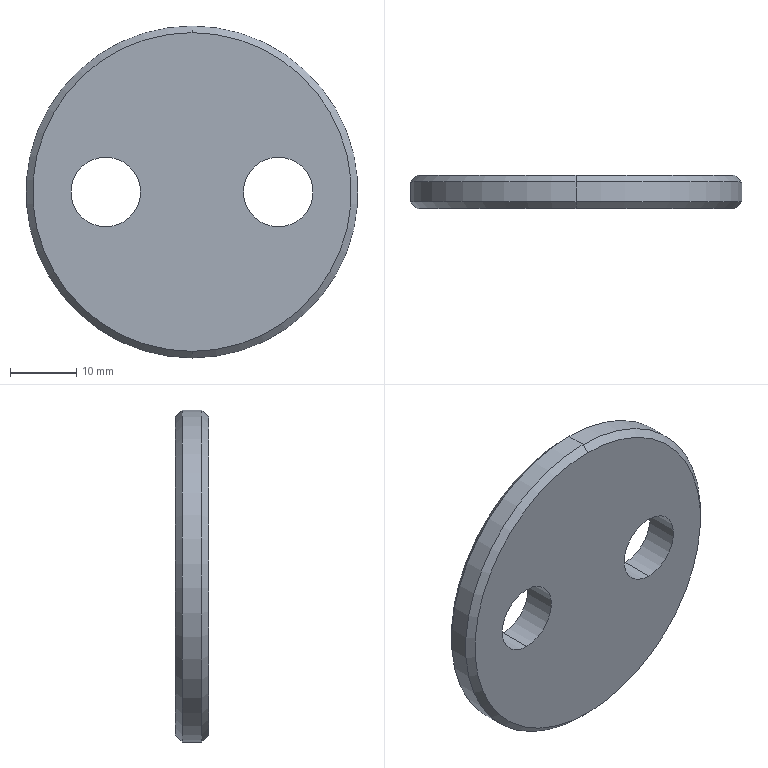Part | SolidWorks | features Chamfer 1, Extrusion 1 | 1 solid | 12 faces | box 50 x 5 x 50 mm | volume 8797 mm3 | cylinder 6 | cone 4 | plane 2 | commonest cylinder face diameters 10.5 x4 50 x2
STEP:
#1=CARTESIAN_POINT('',(0.,5.,24.));
#2=VERTEX_POINT('',#1);
#3=CARTESIAN_POINT('',(0.,5.,-24.));
#4=VERTEX_POINT('',#3);
#5=CARTESIAN_POINT('',(0.,5.,0.));
#6=DIRECTION('',(0.,1.,0.));
#7=DIRECTION('',(0.,0.,1.));
#8=AXIS2_PLACEMENT_3D('',#5,#6,#7);
#9=CIRCLE('',#8,24.);
#10=EDGE_CURVE('',#2,#4,#9,.T.);
#11=ORIENTED_EDGE('',*,*,#10,.F.);
#12=CARTESIAN_POINT('',(0.,4.,25.));
#13=VERTEX_POINT('',#12);
#14=CARTESIAN_POINT('',(0.,5.,24.));
#15=DIRECTION('',(0.,-0.7071,0.7071));
#16=VECTOR('',#15,1000.);
#17=LINE('',#14,#16);
#18=EDGE_CURVE('',#2,#13,#17,.T.);
#19=ORIENTED_EDGE('',*,*,#18,.T.);
#20=CARTESIAN_POINT('',(0.,4.,-25.));
#21=VERTEX_POINT('',#20);
#22=CARTESIAN_POINT('',(0.,4.,0.));
#23=DIRECTION('',(0.,-1.,0.));
#24=DIRECTION('',(0.,0.,1.));
#25=AXIS2_PLACEMENT_3D('',#22,#23,#24);
#26=CIRCLE('',#25,25.);
#27=EDGE_CURVE('',#21,#13,#26,.T.);
#28=ORIENTED_EDGE('',*,*,#27,.F.);
#29=CARTESIAN_POINT('',(0.,5.,-24.));
#30=DIRECTION('',(0.,-0.7071,-0.7071));
#31=VECTOR('',#30,1000.);
#32=LINE('',#29,#31);
#33=EDGE_CURVE('',#4,#21,#32,.T.);
#34=ORIENTED_EDGE('',*,*,#33,.F.);
#35=EDGE_LOOP('',(#11,#19,#28,#34));
#36=FACE_OUTER_BOUND('',#35,.T.);
#37=CARTESIAN_POINT('',(0.,5.,0.));
#38=DIRECTION('',(0.,-1.,0.));
#39=DIRECTION('',(0.,0.,-1.));
#40=AXIS2_PLACEMENT_3D('',#37,#38,#39);
#41=CONICAL_SURFACE('',#40,24.,0.7854);
#42=ADVANCED_FACE('',(#36),#41,.T.);
#43=CARTESIAN_POINT('',(0.,0.,-24.));
#44=VERTEX_POINT('',#43);
#45=CARTESIAN_POINT('',(0.,0.,24.));
#46=VERTEX_POINT('',#45);
#47=CARTESIAN_POINT('',(0.,0.,0.));
#48=DIRECTION('',(0.,-1.,0.));
#49=DIRECTION('',(0.,0.,1.));
#50=AXIS2_PLACEMENT_3D('',#47,#48,#49);
#51=CIRCLE('',#50,24.);
#52=EDGE_CURVE('',#44,#46,#51,.T.);
#53=ORIENTED_EDGE('',*,*,#52,.F.);
#54=CARTESIAN_POINT('',(0.,1.,-25.));
#55=VERTEX_POINT('',#54);
#56=CARTESIAN_POINT('',(0.,1.,-25.));
#57=DIRECTION('',(0.,0.7071,-0.7071));
#58=VECTOR('',#57,1000.);
#59=LINE('',#56,#58);
#60=EDGE_CURVE('',#44,#55,#59,.T.);
#61=ORIENTED_EDGE('',*,*,#60,.T.);
#62=CARTESIAN_POINT('',(0.,1.,25.));
#63=VERTEX_POINT('',#62);
#64=CARTESIAN_POINT('',(0.,1.,0.));
#65=DIRECTION('',(0.,1.,0.));
#66=DIRECTION('',(0.,0.,1.));
#67=AXIS2_PLACEMENT_3D('',#64,#65,#66);
#68=CIRCLE('',#67,25.);
#69=EDGE_CURVE('',#63,#55,#68,.T.);
#70=ORIENTED_EDGE('',*,*,#69,.F.);
#71=CARTESIAN_POINT('',(0.,1.,25.));
#72=DIRECTION('',(0.,0.7071,0.7071));
#73=VECTOR('',#72,1000.);
#74=LINE('',#71,#73);
#75=EDGE_CURVE('',#46,#63,#74,.T.);
#76=ORIENTED_EDGE('',*,*,#75,.F.);
#77=EDGE_LOOP('',(#53,#61,#70,#76));
#78=FACE_OUTER_BOUND('',#77,.T.);
#79=CARTESIAN_POINT('',(0.,1.,0.));
#80=DIRECTION('',(0.,1.,0.));
#81=DIRECTION('',(0.,0.,1.));
#82=AXIS2_PLACEMENT_3D('',#79,#80,#81);
#83=CONICAL_SURFACE('',#82,25.,0.7854);
#84=ADVANCED_FACE('',(#78),#83,.T.);
#85=CARTESIAN_POINT('',(13.,5.,-5.25));
#86=VERTEX_POINT('',#85);
#87=CARTESIAN_POINT('',(13.,5.,5.25));
#88=VERTEX_POINT('',#87);
#89=CARTESIAN_POINT('',(13.,5.,0.));
#90=DIRECTION('',(0.,1.,0.));
#91=DIRECTION('',(0.,0.,-1.));
#92=AXIS2_PLACEMENT_3D('',#89,#90,#91);
#93=CIRCLE('',#92,5.25);
#94=EDGE_CURVE('',#86,#88,#93,.T.);
#95=ORIENTED_EDGE('',*,*,#94,.T.);
#96=CARTESIAN_POINT('',(13.,0.,5.25));
#97=VERTEX_POINT('',#96);
#98=CARTESIAN_POINT('',(13.,5.,5.25));
#99=DIRECTION('',(0.,-1.,0.));
#100=VECTOR('',#99,1000.);
#101=LINE('',#98,#100);
#102=EDGE_CURVE('',#88,#97,#101,.T.);
#103=ORIENTED_EDGE('',*,*,#102,.T.);
#104=CARTESIAN_POINT('',(13.,0.,-5.25));
#105=VERTEX_POINT('',#104);
#106=CARTESIAN_POINT('',(13.,0.,0.));
#107=DIRECTION('',(0.,1.,0.));
#108=DIRECTION('',(0.,0.,-1.));
#109=AXIS2_PLACEMENT_3D('',#106,#107,#108);
#110=CIRCLE('',#109,5.25);
#111=EDGE_CURVE('',#105,#97,#110,.T.);
#112=ORIENTED_EDGE('',*,*,#111,.F.);
#113=CARTESIAN_POINT('',(13.,5.,-5.25));
#114=DIRECTION('',(0.,-1.,0.));
#115=VECTOR('',#114,1000.);
#116=LINE('',#113,#115);
#117=EDGE_CURVE('',#86,#105,#116,.T.);
#118=ORIENTED_EDGE('',*,*,#117,.F.);
#119=EDGE_LOOP('',(#95,#103,#112,#118));
#120=FACE_OUTER_BOUND('',#119,.T.);
#121=CARTESIAN_POINT('',(13.,5.,0.));
#122=DIRECTION('',(0.,-1.,0.));
#123=DIRECTION('',(0.,0.,-1.));
#124=AXIS2_PLACEMENT_3D('',#121,#122,#123);
#125=CYLINDRICAL_SURFACE('',#124,5.25);
#126=ADVANCED_FACE('',(#120),#125,.F.);
#127=CARTESIAN_POINT('',(-13.,5.,-5.25));
#128=VERTEX_POINT('',#127);
#129=CARTESIAN_POINT('',(-13.,5.,5.25));
#130=VERTEX_POINT('',#129);
#131=CARTESIAN_POINT('',(-13.,5.,0.));
#132=DIRECTION('',(0.,1.,0.));
#133=DIRECTION('',(0.,0.,1.));
#134=AXIS2_PLACEMENT_3D('',#131,#132,#133);
#135=CIRCLE('',#134,5.25);
#136=EDGE_CURVE('',#128,#130,#135,.T.);
#137=ORIENTED_EDGE('',*,*,#136,.T.);
#138=CARTESIAN_POINT('',(-13.,0.,5.25));
#139=VERTEX_POINT('',#138);
#140=CARTESIAN_POINT('',(-13.,5.,5.25));
#141=DIRECTION('',(0.,-1.,0.));
#142=VECTOR('',#141,1000.);
#143=LINE('',#140,#142);
#144=EDGE_CURVE('',#130,#139,#143,.T.);
#145=ORIENTED_EDGE('',*,*,#144,.T.);
#146=CARTESIAN_POINT('',(-13.,0.,-5.25));
#147=VERTEX_POINT('',#146);
#148=CARTESIAN_POINT('',(-13.,0.,0.));
#149=DIRECTION('',(0.,1.,0.));
#150=DIRECTION('',(0.,0.,1.));
#151=AXIS2_PLACEMENT_3D('',#148,#149,#150);
#152=CIRCLE('',#151,5.25);
#153=EDGE_CURVE('',#147,#139,#152,.T.);
#154=ORIENTED_EDGE('',*,*,#153,.F.);
#155=CARTESIAN_POINT('',(-13.,5.,-5.25));
#156=DIRECTION('',(0.,-1.,0.));
#157=VECTOR('',#156,1000.);
#158=LINE('',#155,#157);
#159=EDGE_CURVE('',#128,#147,#158,.T.);
#160=ORIENTED_EDGE('',*,*,#159,.F.);
#161=EDGE_LOOP('',(#137,#145,#154,#160));
#162=FACE_OUTER_BOUND('',#161,.T.);
#163=CARTESIAN_POINT('',(-13.,5.,0.));
#164=DIRECTION('',(0.,-1.,0.));
#165=DIRECTION('',(0.,0.,-1.));
#166=AXIS2_PLACEMENT_3D('',#163,#164,#165);
#167=CYLINDRICAL_SURFACE('',#166,5.25);
#168=ADVANCED_FACE('',(#162),#167,.F.);
#169=ORIENTED_EDGE('',*,*,#27,.T.);
#170=CARTESIAN_POINT('',(0.,5.,25.));
#171=DIRECTION('',(0.,-1.,0.));
#172=VECTOR('',#171,1000.);
#173=LINE('',#170,#172);
#174=EDGE_CURVE('',#13,#63,#173,.T.);
#175=ORIENTED_EDGE('',*,*,#174,.T.);
#176=ORIENTED_EDGE('',*,*,#69,.T.);
#177=CARTESIAN_POINT('',(0.,5.,-25.));
#178=DIRECTION('',(0.,-1.,0.));
#179=VECTOR('',#178,1000.);
#180=LINE('',#177,#179);
#181=EDGE_CURVE('',#21,#55,#180,.T.);
#182=ORIENTED_EDGE('',*,*,#181,.F.);
#183=EDGE_LOOP('',(#169,#175,#176,#182));
#184=FACE_OUTER_BOUND('',#183,.T.);
#185=CARTESIAN_POINT('',(0.,5.,0.));
#186=DIRECTION('',(0.,-1.,0.));
#187=DIRECTION('',(0.,0.,-1.));
#188=AXIS2_PLACEMENT_3D('',#185,#186,#187);
#189=CYLINDRICAL_SURFACE('',#188,25.);
#190=ADVANCED_FACE('',(#184),#189,.T.);
#191=CARTESIAN_POINT('',(0.,5.,0.));
#192=DIRECTION('',(0.,1.,0.));
#193=DIRECTION('',(0.,0.,1.));
#194=AXIS2_PLACEMENT_3D('',#191,#192,#193);
#195=CIRCLE('',#194,24.);
#196=EDGE_CURVE('',#4,#2,#195,.T.);
#197=ORIENTED_EDGE('',*,*,#196,.T.);
#198=ORIENTED_EDGE('',*,*,#10,.T.);
#199=EDGE_LOOP('',(#197,#198));
#200=FACE_OUTER_BOUND('',#199,.T.);
#201=ORIENTED_EDGE('',*,*,#136,.F.);
#202=CARTESIAN_POINT('',(-13.,5.,0.));
#203=DIRECTION('',(0.,1.,0.));
#204=DIRECTION('',(0.,0.,1.));
#205=AXIS2_PLACEMENT_3D('',#202,#203,#204);
#206=CIRCLE('',#205,5.25);
#207=EDGE_CURVE('',#130,#128,#206,.T.);
#208=ORIENTED_EDGE('',*,*,#207,.F.);
#209=EDGE_LOOP('',(#201,#208));
#210=FACE_BOUND('',#209,.T.);
#211=ORIENTED_EDGE('',*,*,#94,.F.);
#212=CARTESIAN_POINT('',(13.,5.,0.));
#213=DIRECTION('',(0.,1.,0.));
#214=DIRECTION('',(0.,0.,-1.));
#215=AXIS2_PLACEMENT_3D('',#212,#213,#214);
#216=CIRCLE('',#215,5.25);
#217=EDGE_CURVE('',#88,#86,#216,.T.);
#218=ORIENTED_EDGE('',*,*,#217,.F.);
#219=EDGE_LOOP('',(#211,#218));
#220=FACE_BOUND('',#219,.T.);
#221=CARTESIAN_POINT('',(0.,5.,0.));
#222=DIRECTION('',(0.,1.,0.));
#223=DIRECTION('',(0.,0.,1.));
#224=AXIS2_PLACEMENT_3D('',#221,#222,#223);
#225=PLANE('',#224);
#226=ADVANCED_FACE('',(#200,#210,#220),#225,.T.);
#227=CARTESIAN_POINT('',(0.,0.,0.));
#228=DIRECTION('',(0.,-1.,0.));
#229=DIRECTION('',(0.,0.,1.));
#230=AXIS2_PLACEMENT_3D('',#227,#228,#229);
#231=CIRCLE('',#230,24.);
#232=EDGE_CURVE('',#46,#44,#231,.T.);
#233=ORIENTED_EDGE('',*,*,#232,.T.);
#234=ORIENTED_EDGE('',*,*,#52,.T.);
#235=EDGE_LOOP('',(#233,#234));
#236=FACE_OUTER_BOUND('',#235,.T.);
#237=ORIENTED_EDGE('',*,*,#153,.T.);
#238=CARTESIAN_POINT('',(-13.,0.,0.));
#239=DIRECTION('',(0.,1.,0.));
#240=DIRECTION('',(0.,0.,1.));
#241=AXIS2_PLACEMENT_3D('',#238,#239,#240);
#242=CIRCLE('',#241,5.25);
#243=EDGE_CURVE('',#139,#147,#242,.T.);
#244=ORIENTED_EDGE('',*,*,#243,.T.);
#245=EDGE_LOOP('',(#237,#244));
#246=FACE_BOUND('',#245,.T.);
#247=ORIENTED_EDGE('',*,*,#111,.T.);
#248=CARTESIAN_POINT('',(13.,0.,0.));
#249=DIRECTION('',(0.,1.,0.));
#250=DIRECTION('',(0.,0.,-1.));
#251=AXIS2_PLACEMENT_3D('',#248,#249,#250);
#252=CIRCLE('',#251,5.25);
#253=EDGE_CURVE('',#97,#105,#252,.T.);
#254=ORIENTED_EDGE('',*,*,#253,.T.);
#255=EDGE_LOOP('',(#247,#254));
#256=FACE_BOUND('',#255,.T.);
#257=CARTESIAN_POINT('',(0.,0.,0.));
#258=DIRECTION('',(0.,1.,0.));
#259=DIRECTION('',(0.,0.,1.));
#260=AXIS2_PLACEMENT_3D('',#257,#258,#259);
#261=PLANE('',#260);
#262=ADVANCED_FACE('',(#236,#246,#256),#261,.F.);
#263=ORIENTED_EDGE('',*,*,#174,.F.);
#264=CARTESIAN_POINT('',(0.,4.,0.));
#265=DIRECTION('',(0.,-1.,0.));
#266=DIRECTION('',(0.,0.,1.));
#267=AXIS2_PLACEMENT_3D('',#264,#265,#266);
#268=CIRCLE('',#267,25.);
#269=EDGE_CURVE('',#13,#21,#268,.T.);
#270=ORIENTED_EDGE('',*,*,#269,.T.);
#271=ORIENTED_EDGE('',*,*,#181,.T.);
#272=CARTESIAN_POINT('',(0.,1.,0.));
#273=DIRECTION('',(0.,1.,0.));
#274=DIRECTION('',(0.,0.,1.));
#275=AXIS2_PLACEMENT_3D('',#272,#273,#274);
#276=CIRCLE('',#275,25.);
#277=EDGE_CURVE('',#55,#63,#276,.T.);
#278=ORIENTED_EDGE('',*,*,#277,.T.);
#279=EDGE_LOOP('',(#263,#270,#271,#278));
#280=FACE_OUTER_BOUND('',#279,.T.);
#281=CARTESIAN_POINT('',(0.,5.,0.));
#282=DIRECTION('',(0.,-1.,0.));
#283=DIRECTION('',(0.,0.,-1.));
#284=AXIS2_PLACEMENT_3D('',#281,#282,#283);
#285=CYLINDRICAL_SURFACE('',#284,25.);
#286=ADVANCED_FACE('',(#280),#285,.T.);
#287=ORIENTED_EDGE('',*,*,#144,.F.);
#288=ORIENTED_EDGE('',*,*,#207,.T.);
#289=ORIENTED_EDGE('',*,*,#159,.T.);
#290=ORIENTED_EDGE('',*,*,#243,.F.);
#291=EDGE_LOOP('',(#287,#288,#289,#290));
#292=FACE_OUTER_BOUND('',#291,.T.);
#293=CARTESIAN_POINT('',(-13.,5.,0.));
#294=DIRECTION('',(0.,-1.,0.));
#295=DIRECTION('',(0.,0.,-1.));
#296=AXIS2_PLACEMENT_3D('',#293,#294,#295);
#297=CYLINDRICAL_SURFACE('',#296,5.25);
#298=ADVANCED_FACE('',(#292),#297,.F.);
#299=ORIENTED_EDGE('',*,*,#102,.F.);
#300=ORIENTED_EDGE('',*,*,#217,.T.);
#301=ORIENTED_EDGE('',*,*,#117,.T.);
#302=ORIENTED_EDGE('',*,*,#253,.F.);
#303=EDGE_LOOP('',(#299,#300,#301,#302));
#304=FACE_OUTER_BOUND('',#303,.T.);
#305=CARTESIAN_POINT('',(13.,5.,0.));
#306=DIRECTION('',(0.,-1.,0.));
#307=DIRECTION('',(0.,0.,-1.));
#308=AXIS2_PLACEMENT_3D('',#305,#306,#307);
#309=CYLINDRICAL_SURFACE('',#308,5.25);
#310=ADVANCED_FACE('',(#304),#309,.F.);
#311=ORIENTED_EDGE('',*,*,#60,.F.);
#312=ORIENTED_EDGE('',*,*,#232,.F.);
#313=ORIENTED_EDGE('',*,*,#75,.T.);
#314=ORIENTED_EDGE('',*,*,#277,.F.);
#315=EDGE_LOOP('',(#311,#312,#313,#314));
#316=FACE_OUTER_BOUND('',#315,.T.);
#317=CARTESIAN_POINT('',(0.,1.,0.));
#318=DIRECTION('',(0.,1.,0.));
#319=DIRECTION('',(0.,0.,1.));
#320=AXIS2_PLACEMENT_3D('',#317,#318,#319);
#321=CONICAL_SURFACE('',#320,25.,0.7854);
#322=ADVANCED_FACE('',(#316),#321,.T.);
#323=ORIENTED_EDGE('',*,*,#18,.F.);
#324=ORIENTED_EDGE('',*,*,#196,.F.);
#325=ORIENTED_EDGE('',*,*,#33,.T.);
#326=ORIENTED_EDGE('',*,*,#269,.F.);
#327=EDGE_LOOP('',(#323,#324,#325,#326));
#328=FACE_OUTER_BOUND('',#327,.T.);
#329=CARTESIAN_POINT('',(0.,5.,0.));
#330=DIRECTION('',(0.,-1.,0.));
#331=DIRECTION('',(0.,0.,-1.));
#332=AXIS2_PLACEMENT_3D('',#329,#330,#331);
#333=CONICAL_SURFACE('',#332,24.,0.7854);
#334=ADVANCED_FACE('',(#328),#333,.T.);
#335=CLOSED_SHELL('',(#42,#84,#126,#168,#190,#226,#262,#286,#298,#310,#322,#334));
#336=MANIFOLD_SOLID_BREP('',#335);
#337=CARTESIAN_POINT('',(0.,0.,0.));
#338=DIRECTION('',(0.,0.,1.));
#339=DIRECTION('',(1.,0.,0.));
#340=AXIS2_PLACEMENT_3D('',#337,#338,#339);
#341=(LENGTH_UNIT()NAMED_UNIT(*)SI_UNIT(.MILLI.,.METRE.));
#342=UNCERTAINTY_MEASURE_WITH_UNIT(LENGTH_MEASURE(0.00001),#341,'','');
#343=(NAMED_UNIT(*)PLANE_ANGLE_UNIT()SI_UNIT($,.RADIAN.));
#344=(NAMED_UNIT(*)SI_UNIT($,.STERADIAN.)SOLID_ANGLE_UNIT());
#345=(GEOMETRIC_REPRESENTATION_CONTEXT(3)GLOBAL_UNCERTAINTY_ASSIGNED_CONTEXT((#342))GLOBAL_UNIT_ASSIGNED_CONTEXT((#341,#343,#344))REPRESENTATION_CONTEXT('',''));
#346=ADVANCED_BREP_SHAPE_REPRESENTATION('',(#336,#340),#345);